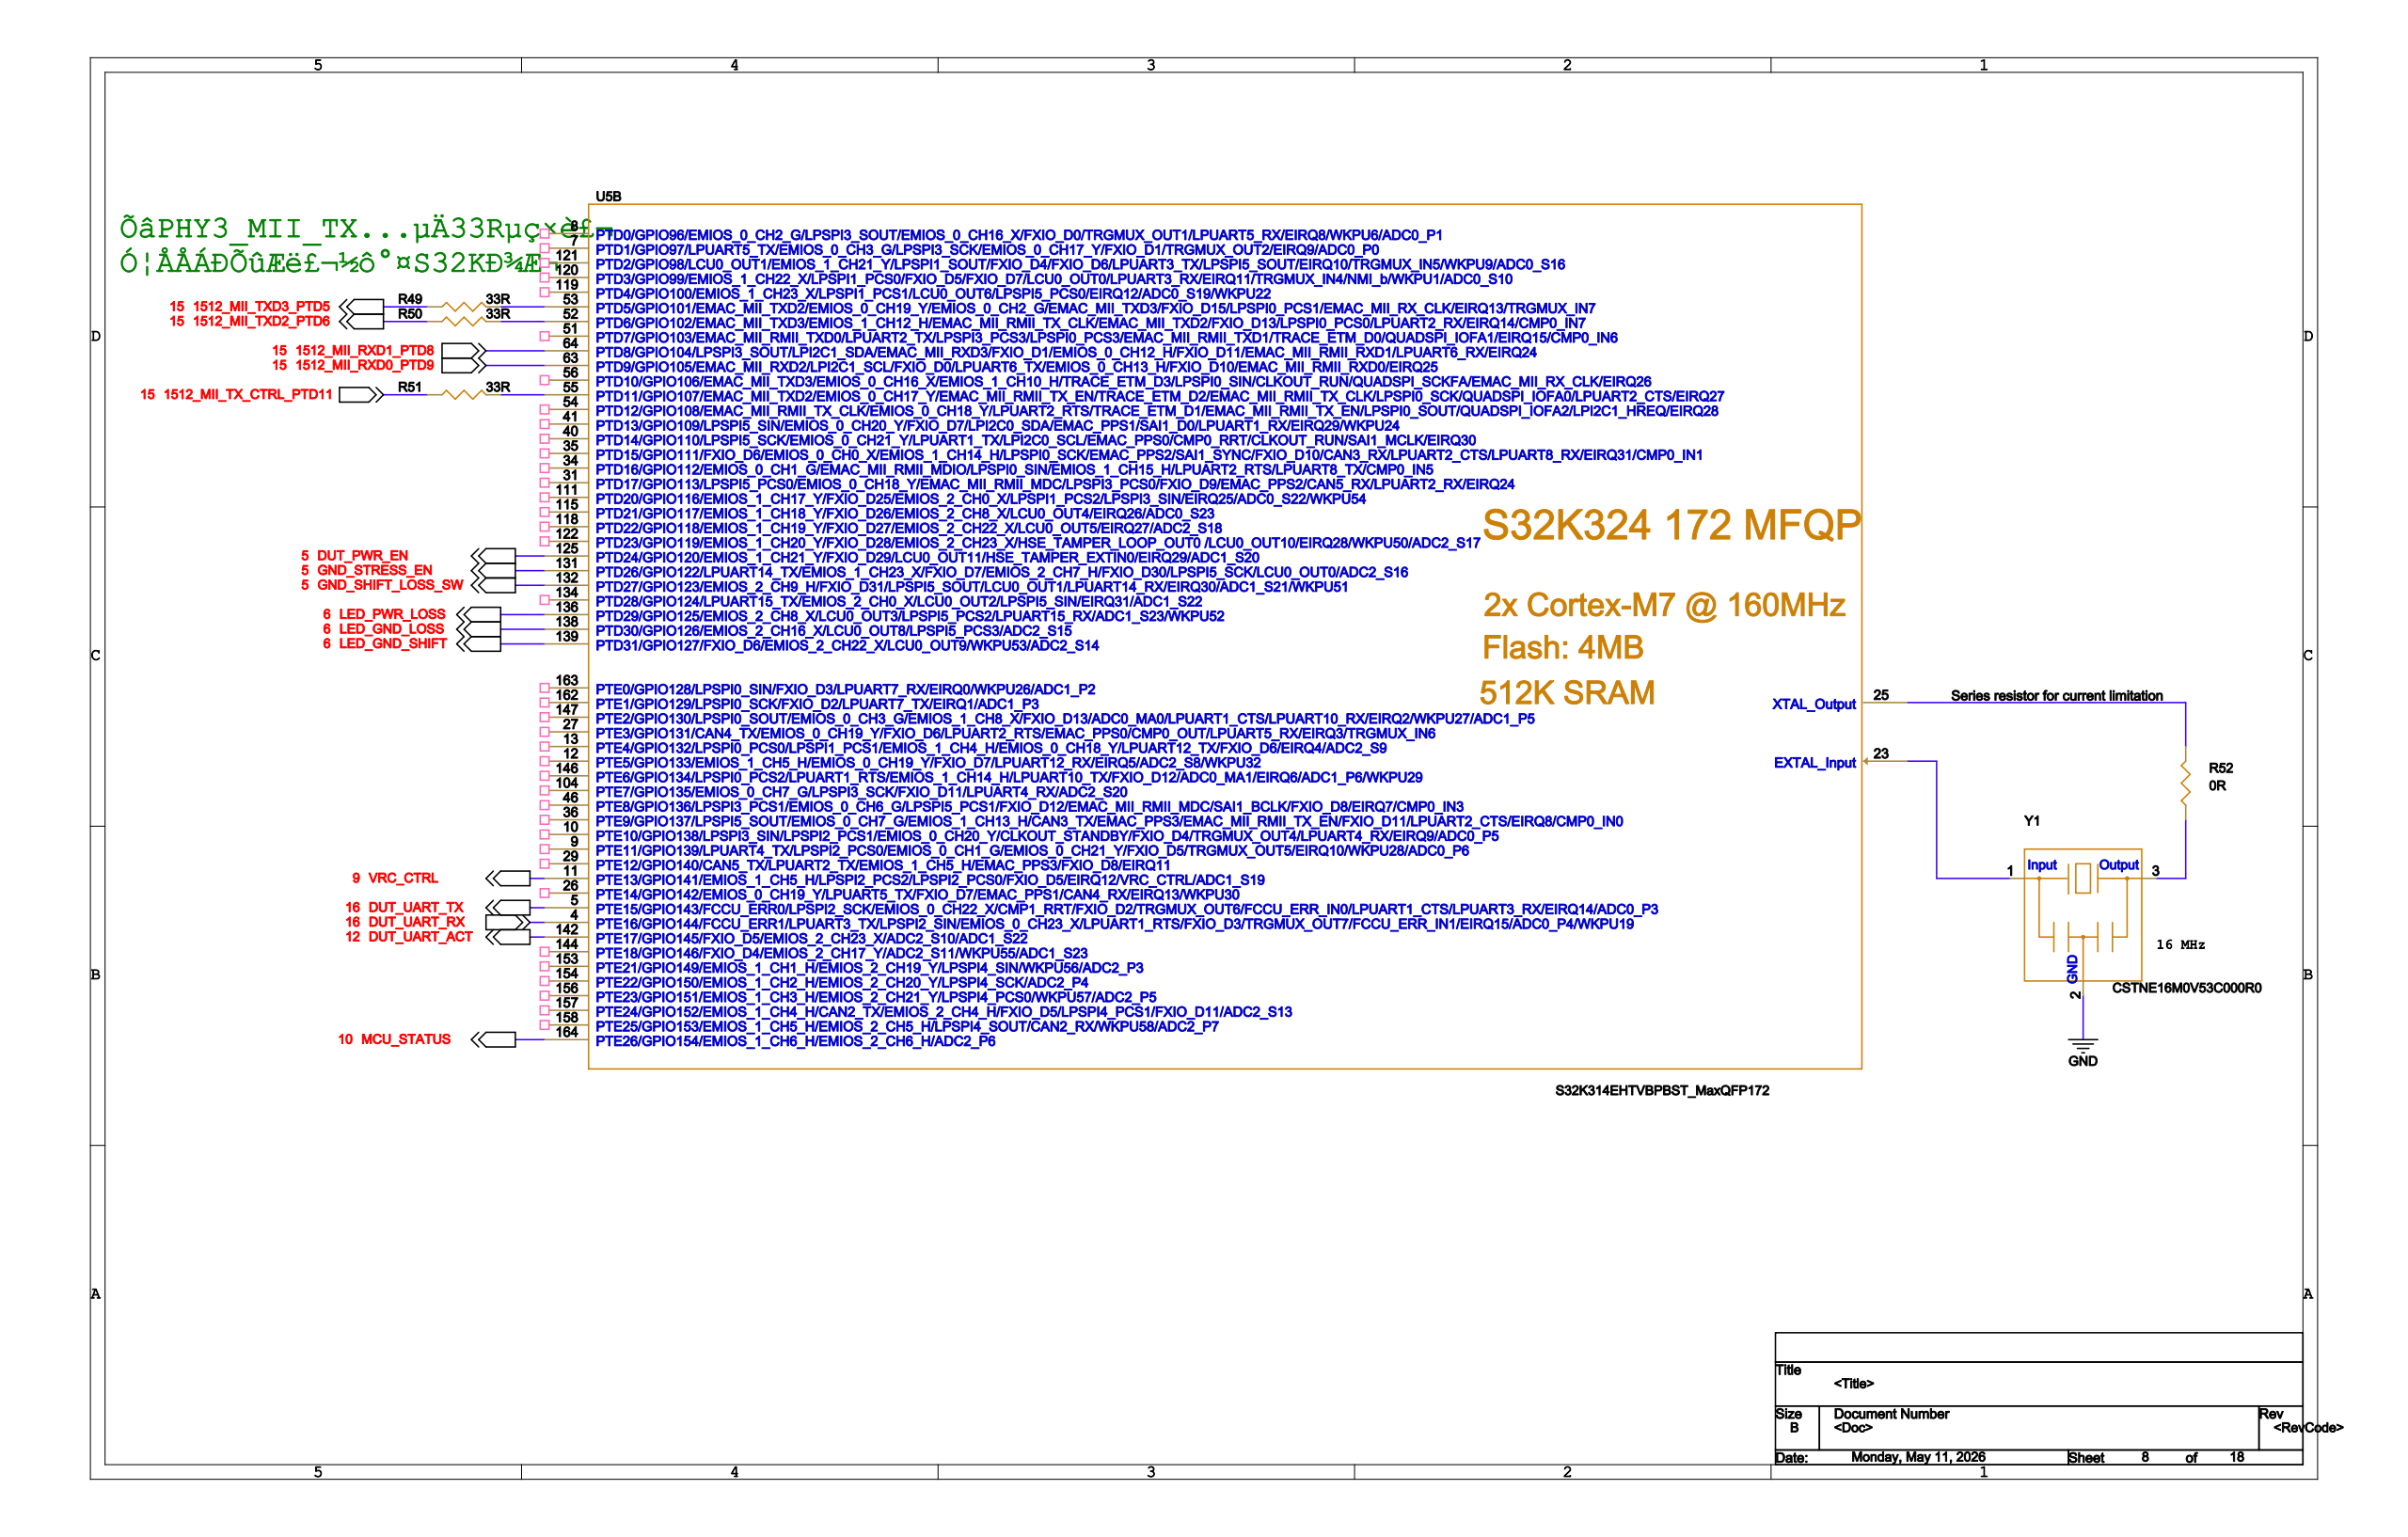Circuit board | Cadence Allegro | 330 parts | 215 nets | one sheet of the schematic
Parts on this sheet (reference | value | footprint):
R49 | 33R | 0402
R50 | 33R | 0402
R51 | 33R | 0402
R52 | 0R | 0402
U5 | S32K314EHTVBPBST_MaxQFP172 | MQFP172_0P65_16X16
Y1 | CSTNE16M0V53C000R0 | CSTNE16M0V53C000R0
Nets of these parts (net: part-pin ...):
GND: Y1-2
DUT_UART_RX: U5-4
DUT_UART_TX: U5-5
1512_MII_RXD0_PTD9: U5-63
1512_MII_RXD1_PTD8: U5-64
1512_MII_TXD3_PTD5: R49-1
N2514215: R49-2 U5-53
1512_MII_TXD2_PTD6: R50-1
N2514203: R50-2 U5-52
1512_MII_TX_CTRL_PTD11: R51-1
N2514195: R51-2 U5-55
MCU_STATUS: U5-164
N1671028: R52-1 Y1-3
N1670986: R52-2 U5-25
VRC_CTRL: U5-11
N1670994: Y1-1 U5-23
DUT_PWR_EN: U5-125
GND_STRESS_EN: U5-131
GND_SHIFT_LOSS_SW: U5-132
LED_PWR_LOSS: U5-136
LED_GND_LOSS: U5-138
LED_GND_SHIFT: U5-139
DUT_UART_ACT: U5-142